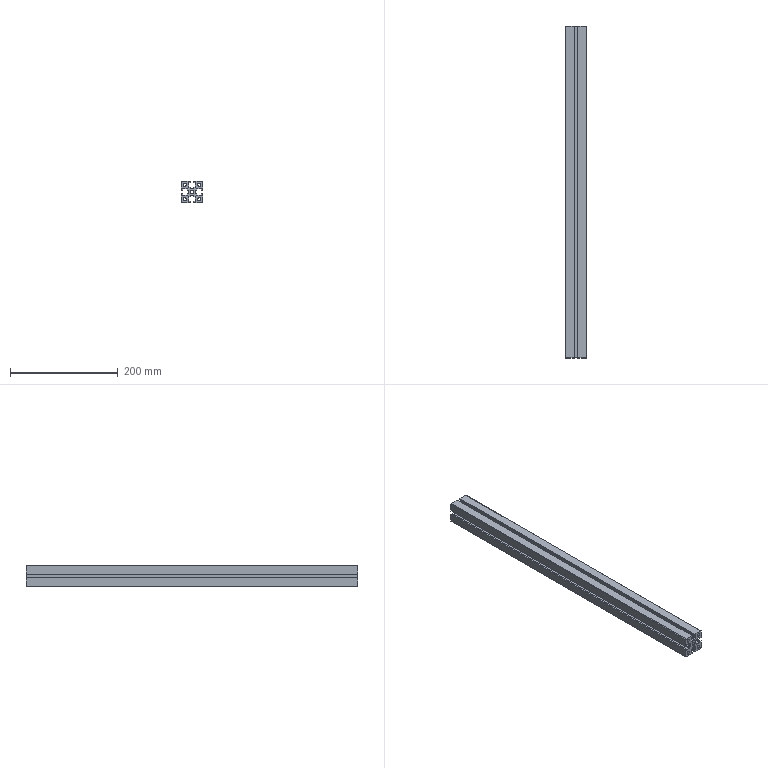Part | STEP file | 01-04 Bracket crossbar 2 | 1 solid | 68 faces | box 40 x 615 x 40 mm | volume 565659 mm3 | plane 54 | cylinder 14 | commonest cylinder face diameters 6 x10 2 x4